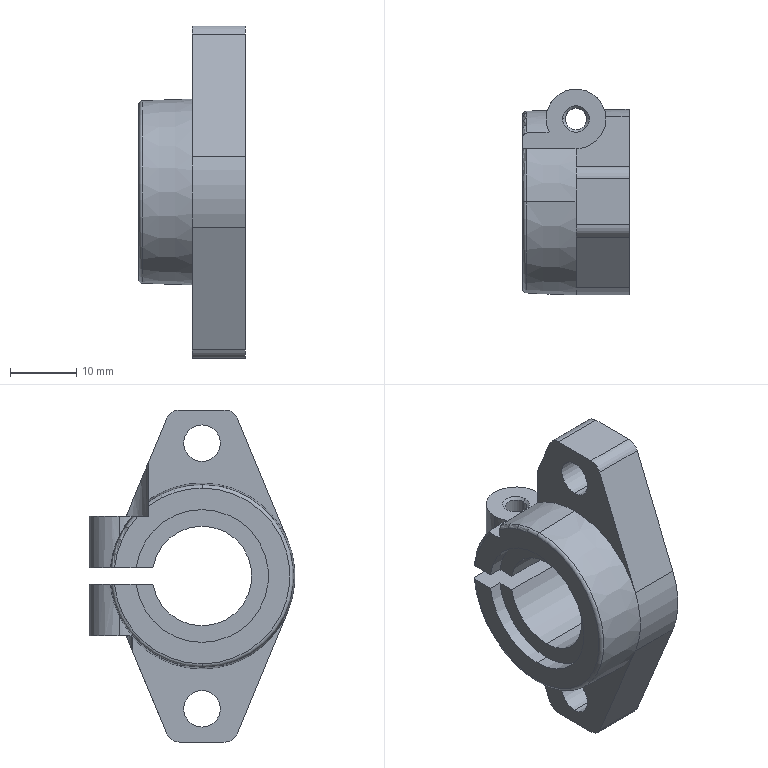Part | SolidWorks | features ICE 5, RefAxis 3, RevCut 3, 3DProfileFeature 1, Extrusion 1, Revolution 1 | 1 solid | 61 faces | box 16 x 31 x 50 mm | volume 9253 mm3 | cylinder 29 | plane 16 | cone 12 | torus 4 | commonest cylinder face diameters 9 x7 3.242 x4 4 x4 5.5 x4 15 x3 20 x3